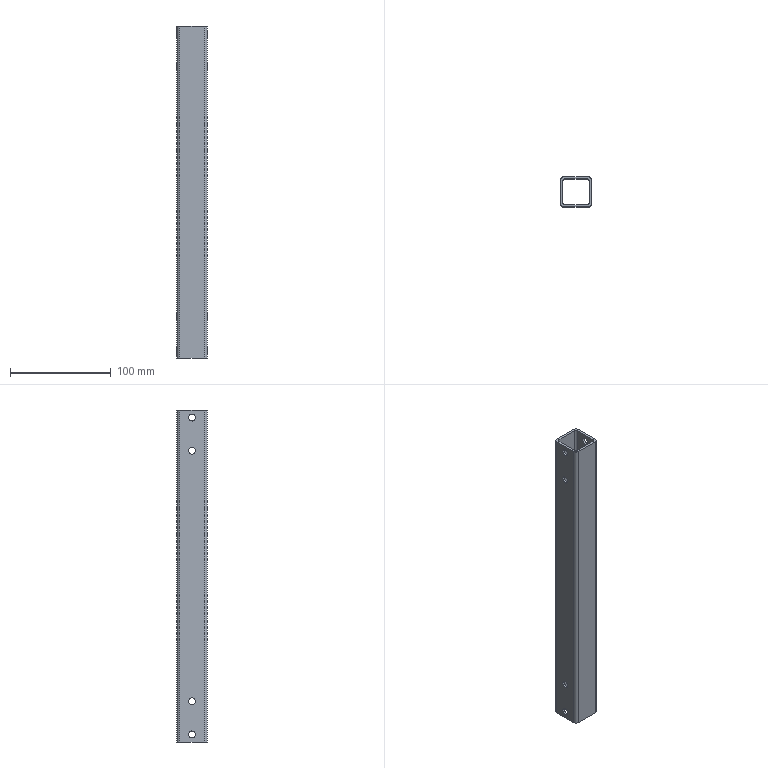Part | STEP file | DIN EN 10210-2 - 20 x 20 x 2 - 300 | 1 solid | 26 faces | box 30 x 30 x 330 mm | volume 71888 mm3 | cylinder 16 | plane 10 | commonest cylinder face diameters 7 x8 4 x4 6 x4